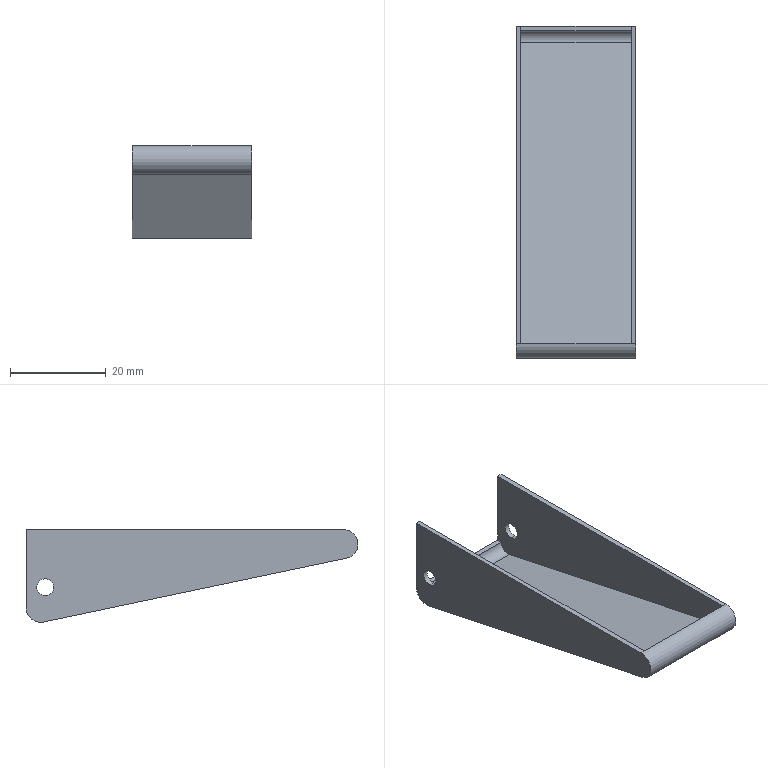Part | SolidWorks | features Extrusion 1, Fillet 1, ICE 1, Shell 1 | 1 solid | 20 faces | box 25 x 69.188 x 19.303 mm | volume 3484 mm3 | plane 12 | cylinder 8 | commonest cylinder face diameters 3.5 x4 4 x2 6 x2
STEP:
#1=CARTESIAN_POINT('',(11.5,91.,-10.25));
#2=VERTEX_POINT('',#1);
#3=CARTESIAN_POINT('',(11.5,91.,-13.75));
#4=VERTEX_POINT('',#3);
#5=CARTESIAN_POINT('',(11.5,91.,-12.));
#6=DIRECTION('',(1.,0.,0.));
#7=DIRECTION('',(0.,0.,-1.));
#8=AXIS2_PLACEMENT_3D('',#5,#6,#7);
#9=CIRCLE('',#8,1.75);
#10=EDGE_CURVE('',#2,#4,#9,.T.);
#11=ORIENTED_EDGE('',*,*,#10,.F.);
#12=CARTESIAN_POINT('',(12.5,91.,-10.25));
#13=VERTEX_POINT('',#12);
#14=CARTESIAN_POINT('',(-12.5,91.,-10.25));
#15=DIRECTION('',(1.,0.,0.));
#16=VECTOR('',#15,1000.);
#17=LINE('',#14,#16);
#18=EDGE_CURVE('',#2,#13,#17,.T.);
#19=ORIENTED_EDGE('',*,*,#18,.T.);
#20=CARTESIAN_POINT('',(12.5,91.,-13.75));
#21=VERTEX_POINT('',#20);
#22=CARTESIAN_POINT('',(12.5,91.,-12.));
#23=DIRECTION('',(1.,0.,0.));
#24=DIRECTION('',(0.,0.,-1.));
#25=AXIS2_PLACEMENT_3D('',#22,#23,#24);
#26=CIRCLE('',#25,1.75);
#27=EDGE_CURVE('',#13,#21,#26,.T.);
#28=ORIENTED_EDGE('',*,*,#27,.T.);
#29=CARTESIAN_POINT('',(-12.5,91.,-13.75));
#30=DIRECTION('',(1.,0.,0.));
#31=VECTOR('',#30,1000.);
#32=LINE('',#29,#31);
#33=EDGE_CURVE('',#4,#21,#32,.T.);
#34=ORIENTED_EDGE('',*,*,#33,.F.);
#35=EDGE_LOOP('',(#11,#19,#28,#34));
#36=FACE_OUTER_BOUND('',#35,.T.);
#37=CARTESIAN_POINT('',(-12.5,91.,-12.));
#38=DIRECTION('',(1.,0.,0.));
#39=DIRECTION('',(0.,0.,-1.));
#40=AXIS2_PLACEMENT_3D('',#37,#38,#39);
#41=CYLINDRICAL_SURFACE('',#40,1.75);
#42=ADVANCED_FACE('',(#36),#41,.F.);
#43=CARTESIAN_POINT('',(-12.5,91.,-10.25));
#44=VERTEX_POINT('',#43);
#45=CARTESIAN_POINT('',(-12.5,91.,-13.75));
#46=VERTEX_POINT('',#45);
#47=CARTESIAN_POINT('',(-12.5,91.,-12.));
#48=DIRECTION('',(1.,0.,0.));
#49=DIRECTION('',(0.,0.,-1.));
#50=AXIS2_PLACEMENT_3D('',#47,#48,#49);
#51=CIRCLE('',#50,1.75);
#52=EDGE_CURVE('',#44,#46,#51,.T.);
#53=ORIENTED_EDGE('',*,*,#52,.F.);
#54=CARTESIAN_POINT('',(-11.5,91.,-10.25));
#55=VERTEX_POINT('',#54);
#56=CARTESIAN_POINT('',(-12.5,91.,-10.25));
#57=DIRECTION('',(1.,0.,0.));
#58=VECTOR('',#57,1000.);
#59=LINE('',#56,#58);
#60=EDGE_CURVE('',#44,#55,#59,.T.);
#61=ORIENTED_EDGE('',*,*,#60,.T.);
#62=CARTESIAN_POINT('',(-11.5,91.,-13.75));
#63=VERTEX_POINT('',#62);
#64=CARTESIAN_POINT('',(-11.5,91.,-12.));
#65=DIRECTION('',(1.,0.,0.));
#66=DIRECTION('',(0.,0.,-1.));
#67=AXIS2_PLACEMENT_3D('',#64,#65,#66);
#68=CIRCLE('',#67,1.75);
#69=EDGE_CURVE('',#55,#63,#68,.T.);
#70=ORIENTED_EDGE('',*,*,#69,.T.);
#71=CARTESIAN_POINT('',(-12.5,91.,-13.75));
#72=DIRECTION('',(1.,0.,0.));
#73=VECTOR('',#72,1000.);
#74=LINE('',#71,#73);
#75=EDGE_CURVE('',#46,#63,#74,.T.);
#76=ORIENTED_EDGE('',*,*,#75,.F.);
#77=EDGE_LOOP('',(#53,#61,#70,#76));
#78=FACE_OUTER_BOUND('',#77,.T.);
#79=CARTESIAN_POINT('',(-12.5,91.,-12.));
#80=DIRECTION('',(1.,0.,0.));
#81=DIRECTION('',(0.,0.,-1.));
#82=AXIS2_PLACEMENT_3D('',#79,#80,#81);
#83=CYLINDRICAL_SURFACE('',#82,1.75);
#84=ADVANCED_FACE('',(#78),#83,.F.);
#85=CARTESIAN_POINT('',(-11.5,95.,-16.303));
#86=VERTEX_POINT('',#85);
#87=CARTESIAN_POINT('',(-11.5,95.,0.));
#88=VERTEX_POINT('',#87);
#89=CARTESIAN_POINT('',(-11.5,95.,0.));
#90=DIRECTION('',(0.,0.,1.));
#91=VECTOR('',#90,1000.);
#92=LINE('',#89,#91);
#93=EDGE_CURVE('',#86,#88,#92,.T.);
#94=ORIENTED_EDGE('',*,*,#93,.F.);
#95=CARTESIAN_POINT('',(-12.5,95.,-16.303));
#96=VERTEX_POINT('',#95);
#97=CARTESIAN_POINT('',(12.5,95.,-16.303));
#98=DIRECTION('',(-1.,0.,0.));
#99=VECTOR('',#98,1000.);
#100=LINE('',#97,#99);
#101=EDGE_CURVE('',#86,#96,#100,.T.);
#102=ORIENTED_EDGE('',*,*,#101,.T.);
#103=CARTESIAN_POINT('',(-12.5,95.,0.));
#104=VERTEX_POINT('',#103);
#105=CARTESIAN_POINT('',(-12.5,95.,0.));
#106=DIRECTION('',(0.,0.,1.));
#107=VECTOR('',#106,1000.);
#108=LINE('',#105,#107);
#109=EDGE_CURVE('',#96,#104,#108,.T.);
#110=ORIENTED_EDGE('',*,*,#109,.T.);
#111=CARTESIAN_POINT('',(12.5,95.,0.));
#112=DIRECTION('',(-1.,0.,0.));
#113=VECTOR('',#112,1000.);
#114=LINE('',#111,#113);
#115=EDGE_CURVE('',#88,#104,#114,.T.);
#116=ORIENTED_EDGE('',*,*,#115,.F.);
#117=EDGE_LOOP('',(#94,#102,#110,#116));
#118=FACE_OUTER_BOUND('',#117,.T.);
#119=CARTESIAN_POINT('',(12.5,95.,0.));
#120=DIRECTION('',(0.,-1.,0.));
#121=DIRECTION('',(0.,0.,-1.));
#122=AXIS2_PLACEMENT_3D('',#119,#120,#121);
#123=PLANE('',#122);
#124=ADVANCED_FACE('',(#118),#123,.F.);
#125=CARTESIAN_POINT('',(-11.5,28.812,0.));
#126=VERTEX_POINT('',#125);
#127=CARTESIAN_POINT('',(-11.5,0.,0.));
#128=DIRECTION('',(0.,-1.,0.));
#129=VECTOR('',#128,1000.);
#130=LINE('',#127,#129);
#131=EDGE_CURVE('',#88,#126,#130,.T.);
#132=ORIENTED_EDGE('',*,*,#131,.F.);
#133=ORIENTED_EDGE('',*,*,#115,.T.);
#134=CARTESIAN_POINT('',(-12.5,28.812,0.));
#135=VERTEX_POINT('',#134);
#136=CARTESIAN_POINT('',(-12.5,0.,0.));
#137=DIRECTION('',(0.,-1.,0.));
#138=VECTOR('',#137,1000.);
#139=LINE('',#136,#138);
#140=EDGE_CURVE('',#104,#135,#139,.T.);
#141=ORIENTED_EDGE('',*,*,#140,.T.);
#142=CARTESIAN_POINT('',(12.5,28.812,0.));
#143=DIRECTION('',(1.,0.,0.));
#144=VECTOR('',#143,1000.);
#145=LINE('',#142,#144);
#146=EDGE_CURVE('',#135,#126,#145,.T.);
#147=ORIENTED_EDGE('',*,*,#146,.T.);
#148=EDGE_LOOP('',(#132,#133,#141,#147));
#149=FACE_OUTER_BOUND('',#148,.T.);
#150=CARTESIAN_POINT('',(12.5,0.,0.));
#151=DIRECTION('',(0.,0.,-1.));
#152=DIRECTION('',(-1.,0.,0.));
#153=AXIS2_PLACEMENT_3D('',#150,#151,#152);
#154=PLANE('',#153);
#155=ADVANCED_FACE('',(#149),#154,.F.);
#156=CARTESIAN_POINT('',(-12.5,28.194,-5.936));
#157=VERTEX_POINT('',#156);
#158=CARTESIAN_POINT('',(-12.5,91.382,-19.238));
#159=VERTEX_POINT('',#158);
#160=CARTESIAN_POINT('',(-12.5,95.,-20.));
#161=DIRECTION('',(0.,0.9785,-0.206));
#162=VECTOR('',#161,1000.);
#163=LINE('',#160,#162);
#164=EDGE_CURVE('',#157,#159,#163,.T.);
#165=ORIENTED_EDGE('',*,*,#164,.T.);
#166=CARTESIAN_POINT('',(12.5,91.382,-19.238));
#167=VERTEX_POINT('',#166);
#168=CARTESIAN_POINT('',(12.5,91.382,-19.238));
#169=DIRECTION('',(1.,0.,0.));
#170=VECTOR('',#169,1000.);
#171=LINE('',#168,#170);
#172=EDGE_CURVE('',#159,#167,#171,.T.);
#173=ORIENTED_EDGE('',*,*,#172,.T.);
#174=CARTESIAN_POINT('',(12.5,28.194,-5.936));
#175=VERTEX_POINT('',#174);
#176=CARTESIAN_POINT('',(12.5,95.,-20.));
#177=DIRECTION('',(0.,0.9785,-0.206));
#178=VECTOR('',#177,1000.);
#179=LINE('',#176,#178);
#180=EDGE_CURVE('',#175,#167,#179,.T.);
#181=ORIENTED_EDGE('',*,*,#180,.F.);
#182=CARTESIAN_POINT('',(12.5,28.194,-5.936));
#183=DIRECTION('',(-1.,0.,0.));
#184=VECTOR('',#183,1000.);
#185=LINE('',#182,#184);
#186=EDGE_CURVE('',#175,#157,#185,.T.);
#187=ORIENTED_EDGE('',*,*,#186,.T.);
#188=EDGE_LOOP('',(#165,#173,#181,#187));
#189=FACE_OUTER_BOUND('',#188,.T.);
#190=CARTESIAN_POINT('',(12.5,95.,-20.));
#191=DIRECTION('',(0.,0.206,0.9785));
#192=DIRECTION('',(0.,-0.9785,0.206));
#193=AXIS2_PLACEMENT_3D('',#190,#191,#192);
#194=PLANE('',#193);
#195=ADVANCED_FACE('',(#189),#194,.F.);
#196=CARTESIAN_POINT('',(12.5,95.,-16.303));
#197=VERTEX_POINT('',#196);
#198=CARTESIAN_POINT('',(11.5,95.,-16.303));
#199=VERTEX_POINT('',#198);
#200=CARTESIAN_POINT('',(12.5,95.,-16.303));
#201=DIRECTION('',(-1.,0.,0.));
#202=VECTOR('',#201,1000.);
#203=LINE('',#200,#202);
#204=EDGE_CURVE('',#197,#199,#203,.T.);
#205=ORIENTED_EDGE('',*,*,#204,.T.);
#206=CARTESIAN_POINT('',(11.5,95.,0.));
#207=VERTEX_POINT('',#206);
#208=CARTESIAN_POINT('',(11.5,95.,0.));
#209=DIRECTION('',(0.,0.,1.));
#210=VECTOR('',#209,1000.);
#211=LINE('',#208,#210);
#212=EDGE_CURVE('',#199,#207,#211,.T.);
#213=ORIENTED_EDGE('',*,*,#212,.T.);
#214=CARTESIAN_POINT('',(12.5,95.,0.));
#215=VERTEX_POINT('',#214);
#216=CARTESIAN_POINT('',(12.5,95.,0.));
#217=DIRECTION('',(-1.,0.,0.));
#218=VECTOR('',#217,1000.);
#219=LINE('',#216,#218);
#220=EDGE_CURVE('',#215,#207,#219,.T.);
#221=ORIENTED_EDGE('',*,*,#220,.F.);
#222=CARTESIAN_POINT('',(12.5,95.,0.));
#223=DIRECTION('',(0.,0.,1.));
#224=VECTOR('',#223,1000.);
#225=LINE('',#222,#224);
#226=EDGE_CURVE('',#197,#215,#225,.T.);
#227=ORIENTED_EDGE('',*,*,#226,.F.);
#228=EDGE_LOOP('',(#205,#213,#221,#227));
#229=FACE_OUTER_BOUND('',#228,.T.);
#230=CARTESIAN_POINT('',(12.5,95.,0.));
#231=DIRECTION('',(0.,-1.,0.));
#232=DIRECTION('',(0.,0.,-1.));
#233=AXIS2_PLACEMENT_3D('',#230,#231,#232);
#234=PLANE('',#233);
#235=ADVANCED_FACE('',(#229),#234,.F.);
#236=ORIENTED_EDGE('',*,*,#220,.T.);
#237=CARTESIAN_POINT('',(11.5,28.812,0.));
#238=VERTEX_POINT('',#237);
#239=CARTESIAN_POINT('',(11.5,0.,0.));
#240=DIRECTION('',(0.,-1.,0.));
#241=VECTOR('',#240,1000.);
#242=LINE('',#239,#241);
#243=EDGE_CURVE('',#207,#238,#242,.T.);
#244=ORIENTED_EDGE('',*,*,#243,.T.);
#245=CARTESIAN_POINT('',(12.5,28.812,0.));
#246=VERTEX_POINT('',#245);
#247=CARTESIAN_POINT('',(12.5,28.812,0.));
#248=DIRECTION('',(1.,0.,0.));
#249=VECTOR('',#248,1000.);
#250=LINE('',#247,#249);
#251=EDGE_CURVE('',#238,#246,#250,.T.);
#252=ORIENTED_EDGE('',*,*,#251,.T.);
#253=CARTESIAN_POINT('',(12.5,0.,0.));
#254=DIRECTION('',(0.,-1.,0.));
#255=VECTOR('',#254,1000.);
#256=LINE('',#253,#255);
#257=EDGE_CURVE('',#215,#246,#256,.T.);
#258=ORIENTED_EDGE('',*,*,#257,.F.);
#259=EDGE_LOOP('',(#236,#244,#252,#258));
#260=FACE_OUTER_BOUND('',#259,.T.);
#261=CARTESIAN_POINT('',(12.5,0.,0.));
#262=DIRECTION('',(0.,0.,-1.));
#263=DIRECTION('',(-1.,0.,0.));
#264=AXIS2_PLACEMENT_3D('',#261,#262,#263);
#265=PLANE('',#264);
#266=ADVANCED_FACE('',(#260),#265,.F.);
#267=CARTESIAN_POINT('',(12.5,91.,-12.));
#268=DIRECTION('',(1.,0.,0.));
#269=DIRECTION('',(0.,0.,-1.));
#270=AXIS2_PLACEMENT_3D('',#267,#268,#269);
#271=CIRCLE('',#270,1.75);
#272=EDGE_CURVE('',#21,#13,#271,.T.);
#273=ORIENTED_EDGE('',*,*,#272,.F.);
#274=ORIENTED_EDGE('',*,*,#27,.F.);
#275=EDGE_LOOP('',(#273,#274));
#276=FACE_BOUND('',#275,.T.);
#277=ORIENTED_EDGE('',*,*,#180,.T.);
#278=CARTESIAN_POINT('',(12.5,92.,-16.303));
#279=DIRECTION('',(1.,0.,0.));
#280=DIRECTION('',(0.,0.,-1.));
#281=AXIS2_PLACEMENT_3D('',#278,#279,#280);
#282=CIRCLE('',#281,3.);
#283=EDGE_CURVE('',#167,#197,#282,.T.);
#284=ORIENTED_EDGE('',*,*,#283,.T.);
#285=ORIENTED_EDGE('',*,*,#226,.T.);
#286=ORIENTED_EDGE('',*,*,#257,.T.);
#287=CARTESIAN_POINT('',(12.5,28.812,-3.));
#288=DIRECTION('',(1.,0.,0.));
#289=DIRECTION('',(0.,0.,-1.));
#290=AXIS2_PLACEMENT_3D('',#287,#288,#289);
#291=CIRCLE('',#290,3.);
#292=EDGE_CURVE('',#246,#175,#291,.T.);
#293=ORIENTED_EDGE('',*,*,#292,.T.);
#294=EDGE_LOOP('',(#277,#284,#285,#286,#293));
#295=FACE_OUTER_BOUND('',#294,.T.);
#296=CARTESIAN_POINT('',(12.5,0.,0.));
#297=DIRECTION('',(1.,0.,0.));
#298=DIRECTION('',(0.,0.,-1.));
#299=AXIS2_PLACEMENT_3D('',#296,#297,#298);
#300=PLANE('',#299);
#301=ADVANCED_FACE('',(#276,#295),#300,.T.);
#302=CARTESIAN_POINT('',(-12.5,91.,-12.));
#303=DIRECTION('',(1.,0.,0.));
#304=DIRECTION('',(0.,0.,-1.));
#305=AXIS2_PLACEMENT_3D('',#302,#303,#304);
#306=CIRCLE('',#305,1.75);
#307=EDGE_CURVE('',#46,#44,#306,.T.);
#308=ORIENTED_EDGE('',*,*,#307,.T.);
#309=ORIENTED_EDGE('',*,*,#52,.T.);
#310=EDGE_LOOP('',(#308,#309));
#311=FACE_BOUND('',#310,.T.);
#312=ORIENTED_EDGE('',*,*,#109,.F.);
#313=CARTESIAN_POINT('',(-12.5,92.,-16.303));
#314=DIRECTION('',(-1.,0.,0.));
#315=DIRECTION('',(0.,0.,-1.));
#316=AXIS2_PLACEMENT_3D('',#313,#314,#315);
#317=CIRCLE('',#316,3.);
#318=EDGE_CURVE('',#96,#159,#317,.T.);
#319=ORIENTED_EDGE('',*,*,#318,.T.);
#320=ORIENTED_EDGE('',*,*,#164,.F.);
#321=CARTESIAN_POINT('',(-12.5,28.812,-3.));
#322=DIRECTION('',(-1.,0.,0.));
#323=DIRECTION('',(0.,0.,-1.));
#324=AXIS2_PLACEMENT_3D('',#321,#322,#323);
#325=CIRCLE('',#324,3.);
#326=EDGE_CURVE('',#157,#135,#325,.T.);
#327=ORIENTED_EDGE('',*,*,#326,.T.);
#328=ORIENTED_EDGE('',*,*,#140,.F.);
#329=EDGE_LOOP('',(#312,#319,#320,#327,#328));
#330=FACE_OUTER_BOUND('',#329,.T.);
#331=CARTESIAN_POINT('',(-12.5,0.,0.));
#332=DIRECTION('',(1.,0.,0.));
#333=DIRECTION('',(0.,0.,-1.));
#334=AXIS2_PLACEMENT_3D('',#331,#332,#333);
#335=PLANE('',#334);
#336=ADVANCED_FACE('',(#311,#330),#335,.F.);
#337=ORIENTED_EDGE('',*,*,#283,.F.);
#338=ORIENTED_EDGE('',*,*,#172,.F.);
#339=ORIENTED_EDGE('',*,*,#318,.F.);
#340=ORIENTED_EDGE('',*,*,#101,.F.);
#341=CARTESIAN_POINT('',(12.5,95.,-16.303));
#342=DIRECTION('',(-1.,0.,0.));
#343=VECTOR('',#342,1000.);
#344=LINE('',#341,#343);
#345=EDGE_CURVE('',#199,#86,#344,.T.);
#346=ORIENTED_EDGE('',*,*,#345,.F.);
#347=ORIENTED_EDGE('',*,*,#204,.F.);
#348=EDGE_LOOP('',(#337,#338,#339,#340,#346,#347));
#349=FACE_OUTER_BOUND('',#348,.T.);
#350=CARTESIAN_POINT('',(12.5,92.,-16.303));
#351=DIRECTION('',(-1.,0.,0.));
#352=DIRECTION('',(0.,0.,1.));
#353=AXIS2_PLACEMENT_3D('',#350,#351,#352);
#354=CYLINDRICAL_SURFACE('',#353,3.);
#355=ADVANCED_FACE('',(#349),#354,.T.);
#356=ORIENTED_EDGE('',*,*,#292,.F.);
#357=ORIENTED_EDGE('',*,*,#251,.F.);
#358=CARTESIAN_POINT('',(12.5,28.812,0.));
#359=DIRECTION('',(1.,0.,0.));
#360=VECTOR('',#359,1000.);
#361=LINE('',#358,#360);
#362=EDGE_CURVE('',#126,#238,#361,.T.);
#363=ORIENTED_EDGE('',*,*,#362,.F.);
#364=ORIENTED_EDGE('',*,*,#146,.F.);
#365=ORIENTED_EDGE('',*,*,#326,.F.);
#366=ORIENTED_EDGE('',*,*,#186,.F.);
#367=EDGE_LOOP('',(#356,#357,#363,#364,#365,#366));
#368=FACE_OUTER_BOUND('',#367,.T.);
#369=CARTESIAN_POINT('',(12.5,28.812,-3.));
#370=DIRECTION('',(-1.,0.,0.));
#371=DIRECTION('',(0.,0.,1.));
#372=AXIS2_PLACEMENT_3D('',#369,#370,#371);
#373=CYLINDRICAL_SURFACE('',#372,3.);
#374=ADVANCED_FACE('',(#368),#373,.T.);
#375=ORIENTED_EDGE('',*,*,#362,.T.);
#376=CARTESIAN_POINT('',(11.5,28.812,-1.));
#377=VERTEX_POINT('',#376);
#378=CARTESIAN_POINT('',(11.5,28.812,0.));
#379=DIRECTION('',(0.,0.,1.));
#380=VECTOR('',#379,1000.);
#381=LINE('',#378,#380);
#382=EDGE_CURVE('',#377,#238,#381,.T.);
#383=ORIENTED_EDGE('',*,*,#382,.F.);
#384=CARTESIAN_POINT('',(-11.5,28.812,-1.));
#385=VERTEX_POINT('',#384);
#386=CARTESIAN_POINT('',(0.,28.812,-1.));
#387=DIRECTION('',(1.,0.,0.));
#388=VECTOR('',#387,1000.);
#389=LINE('',#386,#388);
#390=EDGE_CURVE('',#385,#377,#389,.T.);
#391=ORIENTED_EDGE('',*,*,#390,.F.);
#392=CARTESIAN_POINT('',(-11.5,28.812,0.));
#393=DIRECTION('',(0.,0.,1.));
#394=VECTOR('',#393,1000.);
#395=LINE('',#392,#394);
#396=EDGE_CURVE('',#385,#126,#395,.T.);
#397=ORIENTED_EDGE('',*,*,#396,.T.);
#398=EDGE_LOOP('',(#375,#383,#391,#397));
#399=FACE_OUTER_BOUND('',#398,.T.);
#400=CARTESIAN_POINT('',(12.5,28.812,0.));
#401=DIRECTION('',(0.,-1.,0.));
#402=DIRECTION('',(-1.,0.,0.));
#403=AXIS2_PLACEMENT_3D('',#400,#401,#402);
#404=PLANE('',#403);
#405=ADVANCED_FACE('',(#399),#404,.F.);
#406=ORIENTED_EDGE('',*,*,#345,.T.);
#407=CARTESIAN_POINT('',(-11.5,94.,-16.303));
#408=VERTEX_POINT('',#407);
#409=CARTESIAN_POINT('',(-11.5,95.,-16.303));
#410=DIRECTION('',(0.,1.,0.));
#411=VECTOR('',#410,1000.);
#412=LINE('',#409,#411);
#413=EDGE_CURVE('',#408,#86,#412,.T.);
#414=ORIENTED_EDGE('',*,*,#413,.F.);
#415=CARTESIAN_POINT('',(11.5,94.,-16.303));
#416=VERTEX_POINT('',#415);
#417=CARTESIAN_POINT('',(0.,94.,-16.303));
#418=DIRECTION('',(-1.,0.,0.));
#419=VECTOR('',#418,1000.);
#420=LINE('',#417,#419);
#421=EDGE_CURVE('',#416,#408,#420,.T.);
#422=ORIENTED_EDGE('',*,*,#421,.F.);
#423=CARTESIAN_POINT('',(11.5,95.,-16.303));
#424=DIRECTION('',(0.,1.,0.));
#425=VECTOR('',#424,1000.);
#426=LINE('',#423,#425);
#427=EDGE_CURVE('',#416,#199,#426,.T.);
#428=ORIENTED_EDGE('',*,*,#427,.T.);
#429=EDGE_LOOP('',(#406,#414,#422,#428));
#430=FACE_OUTER_BOUND('',#429,.T.);
#431=CARTESIAN_POINT('',(12.5,95.,-16.303));
#432=DIRECTION('',(0.,0.,1.));
#433=DIRECTION('',(-1.,0.,0.));
#434=AXIS2_PLACEMENT_3D('',#431,#432,#433);
#435=PLANE('',#434);
#436=ADVANCED_FACE('',(#430),#435,.T.);
#437=CARTESIAN_POINT('',(-11.5,28.4,-4.957));
#438=VERTEX_POINT('',#437);
#439=CARTESIAN_POINT('',(-11.5,91.588,-18.26));
#440=VERTEX_POINT('',#439);
#441=CARTESIAN_POINT('',(-11.5,95.206,-19.021));
#442=DIRECTION('',(0.,0.9785,-0.206));
#443=VECTOR('',#442,1000.);
#444=LINE('',#441,#443);
#445=EDGE_CURVE('',#438,#440,#444,.T.);
#446=ORIENTED_EDGE('',*,*,#445,.F.);
#447=CARTESIAN_POINT('',(11.5,28.4,-4.957));
#448=VERTEX_POINT('',#447);
#449=CARTESIAN_POINT('',(12.5,28.4,-4.957));
#450=DIRECTION('',(-1.,0.,0.));
#451=VECTOR('',#450,1000.);
#452=LINE('',#449,#451);
#453=EDGE_CURVE('',#448,#438,#452,.T.);
#454=ORIENTED_EDGE('',*,*,#453,.F.);
#455=CARTESIAN_POINT('',(11.5,91.588,-18.26));
#456=VERTEX_POINT('',#455);
#457=CARTESIAN_POINT('',(11.5,95.206,-19.021));
#458=DIRECTION('',(0.,0.9785,-0.206));
#459=VECTOR('',#458,1000.);
#460=LINE('',#457,#459);
#461=EDGE_CURVE('',#448,#456,#460,.T.);
#462=ORIENTED_EDGE('',*,*,#461,.T.);
#463=CARTESIAN_POINT('',(12.5,91.588,-18.26));
#464=DIRECTION('',(1.,0.,0.));
#465=VECTOR('',#464,1000.);
#466=LINE('',#463,#465);
#467=EDGE_CURVE('',#440,#456,#466,.T.);
#468=ORIENTED_EDGE('',*,*,#467,.F.);
#469=EDGE_LOOP('',(#446,#454,#462,#468));
#470=FACE_OUTER_BOUND('',#469,.T.);
#471=CARTESIAN_POINT('',(12.5,95.206,-19.021));
#472=DIRECTION('',(0.,0.206,0.9785));
#473=DIRECTION('',(0.,-0.9785,0.206));
#474=AXIS2_PLACEMENT_3D('',#471,#472,#473);
#475=PLANE('',#474);
#476=ADVANCED_FACE('',(#470),#475,.T.);
#477=CARTESIAN_POINT('',(11.5,91.,-12.));
#478=DIRECTION('',(1.,0.,0.));
#479=DIRECTION('',(0.,0.,-1.));
#480=AXIS2_PLACEMENT_3D('',#477,#478,#479);
#481=CIRCLE('',#480,1.75);
#482=EDGE_CURVE('',#4,#2,#481,.T.);
#483=ORIENTED_EDGE('',*,*,#482,.T.);
#484=ORIENTED_EDGE('',*,*,#10,.T.);
#485=EDGE_LOOP('',(#483,#484));
#486=FACE_BOUND('',#485,.T.);
#487=ORIENTED_EDGE('',*,*,#461,.F.);
#488=CARTESIAN_POINT('',(11.5,28.812,-3.));
#489=DIRECTION('',(1.,0.,0.));
#490=DIRECTION('',(0.,0.,-1.));
#491=AXIS2_PLACEMENT_3D('',#488,#489,#490);
#492=CIRCLE('',#491,2.);
#493=EDGE_CURVE('',#377,#448,#492,.T.);
#494=ORIENTED_EDGE('',*,*,#493,.F.);
#495=ORIENTED_EDGE('',*,*,#382,.T.);
#496=ORIENTED_EDGE('',*,*,#243,.F.);
#497=ORIENTED_EDGE('',*,*,#212,.F.);
#498=ORIENTED_EDGE('',*,*,#427,.F.);
#499=CARTESIAN_POINT('',(11.5,92.,-16.303));
#500=DIRECTION('',(1.,0.,0.));
#501=DIRECTION('',(0.,0.,-1.));
#502=AXIS2_PLACEMENT_3D('',#499,#500,#501);
#503=CIRCLE('',#502,2.);
#504=EDGE_CURVE('',#456,#416,#503,.T.);
#505=ORIENTED_EDGE('',*,*,#504,.F.);
#506=EDGE_LOOP('',(#487,#494,#495,#496,#497,#498,#505));
#507=FACE_OUTER_BOUND('',#506,.T.);
#508=CARTESIAN_POINT('',(11.5,0.,0.));
#509=DIRECTION('',(1.,0.,0.));
#510=DIRECTION('',(0.,0.,-1.));
#511=AXIS2_PLACEMENT_3D('',#508,#509,#510);
#512=PLANE('',#511);
#513=ADVANCED_FACE('',(#486,#507),#512,.F.);
#514=CARTESIAN_POINT('',(-11.5,91.,-12.));
#515=DIRECTION('',(1.,0.,0.));
#516=DIRECTION('',(0.,0.,-1.));
#517=AXIS2_PLACEMENT_3D('',#514,#515,#516);
#518=CIRCLE('',#517,1.75);
#519=EDGE_CURVE('',#63,#55,#518,.T.);
#520=ORIENTED_EDGE('',*,*,#519,.F.);
#521=ORIENTED_EDGE('',*,*,#69,.F.);
#522=EDGE_LOOP('',(#520,#521));
#523=FACE_BOUND('',#522,.T.);
#524=ORIENTED_EDGE('',*,*,#93,.T.);
#525=ORIENTED_EDGE('',*,*,#131,.T.);
#526=ORIENTED_EDGE('',*,*,#396,.F.);
#527=CARTESIAN_POINT('',(-11.5,28.812,-3.));
#528=DIRECTION('',(-1.,0.,0.));
#529=DIRECTION('',(0.,0.,-1.));
#530=AXIS2_PLACEMENT_3D('',#527,#528,#529);
#531=CIRCLE('',#530,2.);
#532=EDGE_CURVE('',#438,#385,#531,.T.);
#533=ORIENTED_EDGE('',*,*,#532,.F.);
#534=ORIENTED_EDGE('',*,*,#445,.T.);
#535=CARTESIAN_POINT('',(-11.5,92.,-16.303));
#536=DIRECTION('',(-1.,0.,0.));
#537=DIRECTION('',(0.,0.,-1.));
#538=AXIS2_PLACEMENT_3D('',#535,#536,#537);
#539=CIRCLE('',#538,2.);
#540=EDGE_CURVE('',#408,#440,#539,.T.);
#541=ORIENTED_EDGE('',*,*,#540,.F.);
#542=ORIENTED_EDGE('',*,*,#413,.T.);
#543=EDGE_LOOP('',(#524,#525,#526,#533,#534,#541,#542));
#544=FACE_OUTER_BOUND('',#543,.T.);
#545=CARTESIAN_POINT('',(-11.5,0.,0.));
#546=DIRECTION('',(1.,0.,0.));
#547=DIRECTION('',(0.,0.,-1.));
#548=AXIS2_PLACEMENT_3D('',#545,#546,#547);
#549=PLANE('',#548);
#550=ADVANCED_FACE('',(#523,#544),#549,.T.);
#551=ORIENTED_EDGE('',*,*,#504,.T.);
#552=ORIENTED_EDGE('',*,*,#421,.T.);
#553=ORIENTED_EDGE('',*,*,#540,.T.);
#554=ORIENTED_EDGE('',*,*,#467,.T.);
#555=EDGE_LOOP('',(#551,#552,#553,#554));
#556=FACE_OUTER_BOUND('',#555,.T.);
#557=CARTESIAN_POINT('',(12.5,92.,-16.303));
#558=DIRECTION('',(-1.,0.,0.));
#559=DIRECTION('',(0.,0.,1.));
#560=AXIS2_PLACEMENT_3D('',#557,#558,#559);
#561=CYLINDRICAL_SURFACE('',#560,2.);
#562=ADVANCED_FACE('',(#556),#561,.F.);
#563=ORIENTED_EDGE('',*,*,#493,.T.);
#564=ORIENTED_EDGE('',*,*,#453,.T.);
#565=ORIENTED_EDGE('',*,*,#532,.T.);
#566=ORIENTED_EDGE('',*,*,#390,.T.);
#567=EDGE_LOOP('',(#563,#564,#565,#566));
#568=FACE_OUTER_BOUND('',#567,.T.);
#569=CARTESIAN_POINT('',(12.5,28.812,-3.));
#570=DIRECTION('',(-1.,0.,0.));
#571=DIRECTION('',(0.,0.,1.));
#572=AXIS2_PLACEMENT_3D('',#569,#570,#571);
#573=CYLINDRICAL_SURFACE('',#572,2.);
#574=ADVANCED_FACE('',(#568),#573,.F.);
#575=ORIENTED_EDGE('',*,*,#60,.F.);
#576=ORIENTED_EDGE('',*,*,#307,.F.);
#577=ORIENTED_EDGE('',*,*,#75,.T.);
#578=ORIENTED_EDGE('',*,*,#519,.T.);
#579=EDGE_LOOP('',(#575,#576,#577,#578));
#580=FACE_OUTER_BOUND('',#579,.T.);
#581=CARTESIAN_POINT('',(-12.5,91.,-12.));
#582=DIRECTION('',(1.,0.,0.));
#583=DIRECTION('',(0.,0.,-1.));
#584=AXIS2_PLACEMENT_3D('',#581,#582,#583);
#585=CYLINDRICAL_SURFACE('',#584,1.75);
#586=ADVANCED_FACE('',(#580),#585,.F.);
#587=ORIENTED_EDGE('',*,*,#18,.F.);
#588=ORIENTED_EDGE('',*,*,#482,.F.);
#589=ORIENTED_EDGE('',*,*,#33,.T.);
#590=ORIENTED_EDGE('',*,*,#272,.T.);
#591=EDGE_LOOP('',(#587,#588,#589,#590));
#592=FACE_OUTER_BOUND('',#591,.T.);
#593=CARTESIAN_POINT('',(-12.5,91.,-12.));
#594=DIRECTION('',(1.,0.,0.));
#595=DIRECTION('',(0.,0.,-1.));
#596=AXIS2_PLACEMENT_3D('',#593,#594,#595);
#597=CYLINDRICAL_SURFACE('',#596,1.75);
#598=ADVANCED_FACE('',(#592),#597,.F.);
#599=CLOSED_SHELL('',(#42,#84,#124,#155,#195,#235,#266,#301,#336,#355,#374,#405,#436,#476,#513,#550,#562,#574,#586,#598));
#600=MANIFOLD_SOLID_BREP('',#599);
#601=CARTESIAN_POINT('',(0.,0.,0.));
#602=DIRECTION('',(0.,0.,1.));
#603=DIRECTION('',(1.,0.,0.));
#604=AXIS2_PLACEMENT_3D('',#601,#602,#603);
#605=(LENGTH_UNIT()NAMED_UNIT(*)SI_UNIT(.MILLI.,.METRE.));
#606=UNCERTAINTY_MEASURE_WITH_UNIT(LENGTH_MEASURE(0.00001),#605,'','');
#607=(NAMED_UNIT(*)PLANE_ANGLE_UNIT()SI_UNIT($,.RADIAN.));
#608=(NAMED_UNIT(*)SI_UNIT($,.STERADIAN.)SOLID_ANGLE_UNIT());
#609=(GEOMETRIC_REPRESENTATION_CONTEXT(3)GLOBAL_UNCERTAINTY_ASSIGNED_CONTEXT((#606))GLOBAL_UNIT_ASSIGNED_CONTEXT((#605,#607,#608))REPRESENTATION_CONTEXT('',''));
#610=ADVANCED_BREP_SHAPE_REPRESENTATION('',(#600,#604),#609);